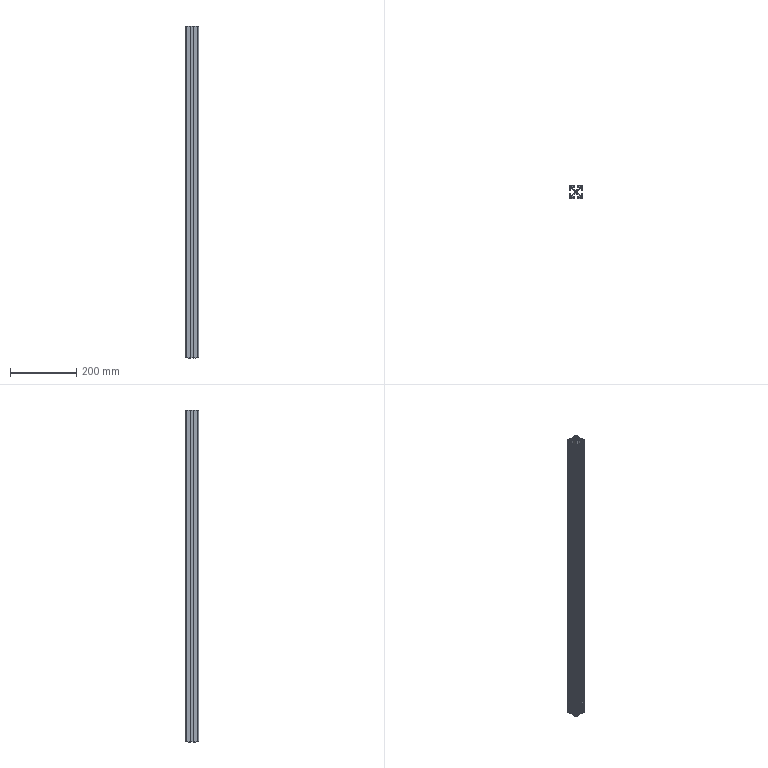Part | STEP file | LE-8-4040-S-OO_LE0311094946 | 1 solid | 188 faces | box 40 x 40 x 1000 mm | volume 478249 mm3 | cylinder 94 | plane 94 | commonest cylinder face diameters 0.6 x30 2 x28 4 x16 0.4 x8 6 x4 9 x4